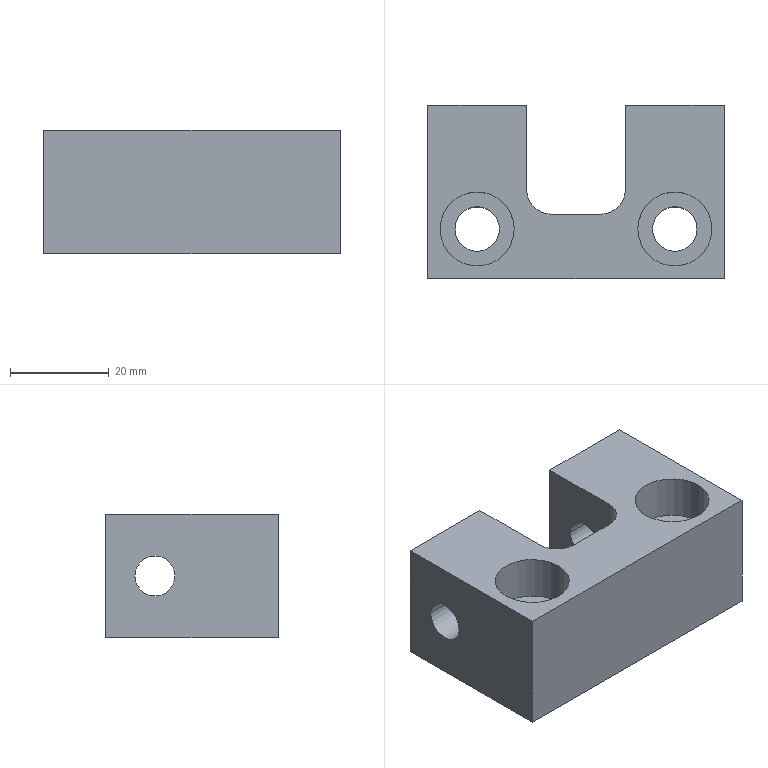Part | SolidWorks | features BaseBody 1 | 1 solid | 26 faces | box 60 x 35 x 25 mm | volume 34490 mm3 | cylinder 14 | plane 12 | commonest cylinder face diameters 8.1 x4 9 x4 15 x4 10 x2
STEP:
#1=CARTESIAN_POINT('',(-27.5,-7.5,16.));
#2=VERTEX_POINT('',#1);
#3=CARTESIAN_POINT('',(-12.5,-7.5,16.));
#4=VERTEX_POINT('',#3);
#5=CARTESIAN_POINT('',(-20.,-7.5,16.));
#6=DIRECTION('',(0.,0.,1.));
#7=DIRECTION('',(1.,0.,0.));
#8=AXIS2_PLACEMENT_3D('',#5,#6,#7);
#9=CIRCLE('',#8,7.5);
#10=EDGE_CURVE('',#2,#4,#9,.T.);
#11=ORIENTED_EDGE('',*,*,#10,.F.);
#12=CARTESIAN_POINT('',(-27.5,-7.5,25.));
#13=VERTEX_POINT('',#12);
#14=CARTESIAN_POINT('',(-27.5,-7.5,25.));
#15=DIRECTION('',(0.,0.,1.));
#16=VECTOR('',#15,1000.);
#17=LINE('',#14,#16);
#18=EDGE_CURVE('',#2,#13,#17,.T.);
#19=ORIENTED_EDGE('',*,*,#18,.T.);
#20=CARTESIAN_POINT('',(-12.5,-7.5,25.));
#21=VERTEX_POINT('',#20);
#22=CARTESIAN_POINT('',(-20.,-7.5,25.));
#23=DIRECTION('',(0.,0.,1.));
#24=DIRECTION('',(1.,0.,0.));
#25=AXIS2_PLACEMENT_3D('',#22,#23,#24);
#26=CIRCLE('',#25,7.5);
#27=EDGE_CURVE('',#13,#21,#26,.T.);
#28=ORIENTED_EDGE('',*,*,#27,.T.);
#29=CARTESIAN_POINT('',(-12.5,-7.5,25.));
#30=DIRECTION('',(0.,0.,1.));
#31=VECTOR('',#30,1000.);
#32=LINE('',#29,#31);
#33=EDGE_CURVE('',#4,#21,#32,.T.);
#34=ORIENTED_EDGE('',*,*,#33,.F.);
#35=EDGE_LOOP('',(#11,#19,#28,#34));
#36=FACE_OUTER_BOUND('',#35,.T.);
#37=CARTESIAN_POINT('',(-20.,-7.5,25.));
#38=DIRECTION('',(0.,0.,1.));
#39=DIRECTION('',(1.,0.,0.));
#40=AXIS2_PLACEMENT_3D('',#37,#38,#39);
#41=CYLINDRICAL_SURFACE('',#40,7.5);
#42=ADVANCED_FACE('',(#36),#41,.F.);
#43=CARTESIAN_POINT('',(-24.5,-7.5,0.));
#44=VERTEX_POINT('',#43);
#45=CARTESIAN_POINT('',(-15.5,-7.5,0.));
#46=VERTEX_POINT('',#45);
#47=CARTESIAN_POINT('',(-20.,-7.5,0.));
#48=DIRECTION('',(0.,0.,1.));
#49=DIRECTION('',(1.,0.,0.));
#50=AXIS2_PLACEMENT_3D('',#47,#48,#49);
#51=CIRCLE('',#50,4.5);
#52=EDGE_CURVE('',#44,#46,#51,.T.);
#53=ORIENTED_EDGE('',*,*,#52,.F.);
#54=CARTESIAN_POINT('',(-24.5,-7.5,16.));
#55=VERTEX_POINT('',#54);
#56=CARTESIAN_POINT('',(-24.5,-7.5,25.));
#57=DIRECTION('',(0.,0.,1.));
#58=VECTOR('',#57,1000.);
#59=LINE('',#56,#58);
#60=EDGE_CURVE('',#44,#55,#59,.T.);
#61=ORIENTED_EDGE('',*,*,#60,.T.);
#62=CARTESIAN_POINT('',(-15.5,-7.5,16.));
#63=VERTEX_POINT('',#62);
#64=CARTESIAN_POINT('',(-20.,-7.5,16.));
#65=DIRECTION('',(0.,0.,1.));
#66=DIRECTION('',(1.,0.,0.));
#67=AXIS2_PLACEMENT_3D('',#64,#65,#66);
#68=CIRCLE('',#67,4.5);
#69=EDGE_CURVE('',#55,#63,#68,.T.);
#70=ORIENTED_EDGE('',*,*,#69,.T.);
#71=CARTESIAN_POINT('',(-15.5,-7.5,25.));
#72=DIRECTION('',(0.,0.,1.));
#73=VECTOR('',#72,1000.);
#74=LINE('',#71,#73);
#75=EDGE_CURVE('',#46,#63,#74,.T.);
#76=ORIENTED_EDGE('',*,*,#75,.F.);
#77=EDGE_LOOP('',(#53,#61,#70,#76));
#78=FACE_OUTER_BOUND('',#77,.T.);
#79=CARTESIAN_POINT('',(-20.,-7.5,25.));
#80=DIRECTION('',(0.,0.,1.));
#81=DIRECTION('',(1.,0.,0.));
#82=AXIS2_PLACEMENT_3D('',#79,#80,#81);
#83=CYLINDRICAL_SURFACE('',#82,4.5);
#84=ADVANCED_FACE('',(#78),#83,.F.);
#85=CARTESIAN_POINT('',(12.5,-7.5,16.));
#86=VERTEX_POINT('',#85);
#87=CARTESIAN_POINT('',(27.5,-7.5,16.));
#88=VERTEX_POINT('',#87);
#89=CARTESIAN_POINT('',(20.,-7.5,16.));
#90=DIRECTION('',(0.,0.,1.));
#91=DIRECTION('',(1.,0.,0.));
#92=AXIS2_PLACEMENT_3D('',#89,#90,#91);
#93=CIRCLE('',#92,7.5);
#94=EDGE_CURVE('',#86,#88,#93,.T.);
#95=ORIENTED_EDGE('',*,*,#94,.F.);
#96=CARTESIAN_POINT('',(12.5,-7.5,25.));
#97=VERTEX_POINT('',#96);
#98=CARTESIAN_POINT('',(12.5,-7.5,25.));
#99=DIRECTION('',(0.,0.,1.));
#100=VECTOR('',#99,1000.);
#101=LINE('',#98,#100);
#102=EDGE_CURVE('',#86,#97,#101,.T.);
#103=ORIENTED_EDGE('',*,*,#102,.T.);
#104=CARTESIAN_POINT('',(27.5,-7.5,25.));
#105=VERTEX_POINT('',#104);
#106=CARTESIAN_POINT('',(20.,-7.5,25.));
#107=DIRECTION('',(0.,0.,1.));
#108=DIRECTION('',(1.,0.,0.));
#109=AXIS2_PLACEMENT_3D('',#106,#107,#108);
#110=CIRCLE('',#109,7.5);
#111=EDGE_CURVE('',#97,#105,#110,.T.);
#112=ORIENTED_EDGE('',*,*,#111,.T.);
#113=CARTESIAN_POINT('',(27.5,-7.5,25.));
#114=DIRECTION('',(0.,0.,1.));
#115=VECTOR('',#114,1000.);
#116=LINE('',#113,#115);
#117=EDGE_CURVE('',#88,#105,#116,.T.);
#118=ORIENTED_EDGE('',*,*,#117,.F.);
#119=EDGE_LOOP('',(#95,#103,#112,#118));
#120=FACE_OUTER_BOUND('',#119,.T.);
#121=CARTESIAN_POINT('',(20.,-7.5,25.));
#122=DIRECTION('',(0.,0.,1.));
#123=DIRECTION('',(1.,0.,0.));
#124=AXIS2_PLACEMENT_3D('',#121,#122,#123);
#125=CYLINDRICAL_SURFACE('',#124,7.5);
#126=ADVANCED_FACE('',(#120),#125,.F.);
#127=CARTESIAN_POINT('',(15.5,-7.5,0.));
#128=VERTEX_POINT('',#127);
#129=CARTESIAN_POINT('',(24.5,-7.5,0.));
#130=VERTEX_POINT('',#129);
#131=CARTESIAN_POINT('',(20.,-7.5,0.));
#132=DIRECTION('',(0.,0.,1.));
#133=DIRECTION('',(1.,0.,0.));
#134=AXIS2_PLACEMENT_3D('',#131,#132,#133);
#135=CIRCLE('',#134,4.5);
#136=EDGE_CURVE('',#128,#130,#135,.T.);
#137=ORIENTED_EDGE('',*,*,#136,.F.);
#138=CARTESIAN_POINT('',(15.5,-7.5,16.));
#139=VERTEX_POINT('',#138);
#140=CARTESIAN_POINT('',(15.5,-7.5,25.));
#141=DIRECTION('',(0.,0.,1.));
#142=VECTOR('',#141,1000.);
#143=LINE('',#140,#142);
#144=EDGE_CURVE('',#128,#139,#143,.T.);
#145=ORIENTED_EDGE('',*,*,#144,.T.);
#146=CARTESIAN_POINT('',(24.5,-7.5,16.));
#147=VERTEX_POINT('',#146);
#148=CARTESIAN_POINT('',(20.,-7.5,16.));
#149=DIRECTION('',(0.,0.,1.));
#150=DIRECTION('',(1.,0.,0.));
#151=AXIS2_PLACEMENT_3D('',#148,#149,#150);
#152=CIRCLE('',#151,4.5);
#153=EDGE_CURVE('',#139,#147,#152,.T.);
#154=ORIENTED_EDGE('',*,*,#153,.T.);
#155=CARTESIAN_POINT('',(24.5,-7.5,25.));
#156=DIRECTION('',(0.,0.,1.));
#157=VECTOR('',#156,1000.);
#158=LINE('',#155,#157);
#159=EDGE_CURVE('',#130,#147,#158,.T.);
#160=ORIENTED_EDGE('',*,*,#159,.F.);
#161=EDGE_LOOP('',(#137,#145,#154,#160));
#162=FACE_OUTER_BOUND('',#161,.T.);
#163=CARTESIAN_POINT('',(20.,-7.5,25.));
#164=DIRECTION('',(0.,0.,1.));
#165=DIRECTION('',(1.,0.,0.));
#166=AXIS2_PLACEMENT_3D('',#163,#164,#165);
#167=CYLINDRICAL_SURFACE('',#166,4.5);
#168=ADVANCED_FACE('',(#162),#167,.F.);
#169=CARTESIAN_POINT('',(-30.,3.45,12.5));
#170=VERTEX_POINT('',#169);
#171=CARTESIAN_POINT('',(-30.,11.55,12.5));
#172=VERTEX_POINT('',#171);
#173=CARTESIAN_POINT('',(-30.,7.5,12.5));
#174=DIRECTION('',(1.,0.,0.));
#175=DIRECTION('',(0.,1.,0.));
#176=AXIS2_PLACEMENT_3D('',#173,#174,#175);
#177=CIRCLE('',#176,4.05);
#178=EDGE_CURVE('',#170,#172,#177,.T.);
#179=ORIENTED_EDGE('',*,*,#178,.F.);
#180=CARTESIAN_POINT('',(-10.,3.45,12.5));
#181=VERTEX_POINT('',#180);
#182=CARTESIAN_POINT('',(-30.,3.45,12.5));
#183=DIRECTION('',(1.,0.,0.));
#184=VECTOR('',#183,1000.);
#185=LINE('',#182,#184);
#186=EDGE_CURVE('',#170,#181,#185,.T.);
#187=ORIENTED_EDGE('',*,*,#186,.T.);
#188=CARTESIAN_POINT('',(-10.,11.55,12.5));
#189=VERTEX_POINT('',#188);
#190=CARTESIAN_POINT('',(-10.,7.5,12.5));
#191=DIRECTION('',(1.,0.,0.));
#192=DIRECTION('',(0.,0.,1.));
#193=AXIS2_PLACEMENT_3D('',#190,#191,#192);
#194=CIRCLE('',#193,4.05);
#195=EDGE_CURVE('',#181,#189,#194,.T.);
#196=ORIENTED_EDGE('',*,*,#195,.T.);
#197=CARTESIAN_POINT('',(-30.,11.55,12.5));
#198=DIRECTION('',(1.,0.,0.));
#199=VECTOR('',#198,1000.);
#200=LINE('',#197,#199);
#201=EDGE_CURVE('',#172,#189,#200,.T.);
#202=ORIENTED_EDGE('',*,*,#201,.F.);
#203=EDGE_LOOP('',(#179,#187,#196,#202));
#204=FACE_OUTER_BOUND('',#203,.T.);
#205=CARTESIAN_POINT('',(-30.,7.5,12.5));
#206=DIRECTION('',(1.,0.,0.));
#207=DIRECTION('',(0.,1.,0.));
#208=AXIS2_PLACEMENT_3D('',#205,#206,#207);
#209=CYLINDRICAL_SURFACE('',#208,4.05);
#210=ADVANCED_FACE('',(#204),#209,.F.);
#211=CARTESIAN_POINT('',(10.,11.55,12.5));
#212=VERTEX_POINT('',#211);
#213=CARTESIAN_POINT('',(10.,3.45,12.5));
#214=VERTEX_POINT('',#213);
#215=CARTESIAN_POINT('',(10.,7.5,12.5));
#216=DIRECTION('',(-1.,0.,0.));
#217=DIRECTION('',(0.,1.,0.));
#218=AXIS2_PLACEMENT_3D('',#215,#216,#217);
#219=CIRCLE('',#218,4.05);
#220=EDGE_CURVE('',#212,#214,#219,.T.);
#221=ORIENTED_EDGE('',*,*,#220,.T.);
#222=CARTESIAN_POINT('',(30.,3.45,12.5));
#223=VERTEX_POINT('',#222);
#224=CARTESIAN_POINT('',(-30.,3.45,12.5));
#225=DIRECTION('',(1.,0.,0.));
#226=VECTOR('',#225,1000.);
#227=LINE('',#224,#226);
#228=EDGE_CURVE('',#214,#223,#227,.T.);
#229=ORIENTED_EDGE('',*,*,#228,.T.);
#230=CARTESIAN_POINT('',(30.,11.55,12.5));
#231=VERTEX_POINT('',#230);
#232=CARTESIAN_POINT('',(30.,7.5,12.5));
#233=DIRECTION('',(1.,0.,0.));
#234=DIRECTION('',(0.,1.,0.));
#235=AXIS2_PLACEMENT_3D('',#232,#233,#234);
#236=CIRCLE('',#235,4.05);
#237=EDGE_CURVE('',#223,#231,#236,.T.);
#238=ORIENTED_EDGE('',*,*,#237,.T.);
#239=CARTESIAN_POINT('',(-30.,11.55,12.5));
#240=DIRECTION('',(1.,0.,0.));
#241=VECTOR('',#240,1000.);
#242=LINE('',#239,#241);
#243=EDGE_CURVE('',#212,#231,#242,.T.);
#244=ORIENTED_EDGE('',*,*,#243,.F.);
#245=EDGE_LOOP('',(#221,#229,#238,#244));
#246=FACE_OUTER_BOUND('',#245,.T.);
#247=CARTESIAN_POINT('',(-30.,7.5,12.5));
#248=DIRECTION('',(1.,0.,0.));
#249=DIRECTION('',(0.,1.,0.));
#250=AXIS2_PLACEMENT_3D('',#247,#248,#249);
#251=CYLINDRICAL_SURFACE('',#250,4.05);
#252=ADVANCED_FACE('',(#246),#251,.F.);
#253=CARTESIAN_POINT('',(-10.,0.5,0.));
#254=VERTEX_POINT('',#253);
#255=CARTESIAN_POINT('',(-5.,-4.5,0.));
#256=VERTEX_POINT('',#255);
#257=CARTESIAN_POINT('',(-5.,0.5,0.));
#258=DIRECTION('',(0.,0.,1.));
#259=DIRECTION('',(1.,0.,0.));
#260=AXIS2_PLACEMENT_3D('',#257,#258,#259);
#261=CIRCLE('',#260,5.);
#262=EDGE_CURVE('',#254,#256,#261,.T.);
#263=ORIENTED_EDGE('',*,*,#262,.F.);
#264=CARTESIAN_POINT('',(-10.,0.5,25.));
#265=VERTEX_POINT('',#264);
#266=CARTESIAN_POINT('',(-10.,0.5,0.));
#267=DIRECTION('',(0.,0.,-1.));
#268=VECTOR('',#267,1000.);
#269=LINE('',#266,#268);
#270=EDGE_CURVE('',#265,#254,#269,.T.);
#271=ORIENTED_EDGE('',*,*,#270,.F.);
#272=CARTESIAN_POINT('',(-5.,-4.5,25.));
#273=VERTEX_POINT('',#272);
#274=CARTESIAN_POINT('',(-5.,0.5,25.));
#275=DIRECTION('',(0.,0.,-1.));
#276=DIRECTION('',(1.,0.,0.));
#277=AXIS2_PLACEMENT_3D('',#274,#275,#276);
#278=CIRCLE('',#277,5.);
#279=EDGE_CURVE('',#273,#265,#278,.T.);
#280=ORIENTED_EDGE('',*,*,#279,.F.);
#281=CARTESIAN_POINT('',(-5.,-4.5,25.));
#282=DIRECTION('',(0.,0.,1.));
#283=VECTOR('',#282,1000.);
#284=LINE('',#281,#283);
#285=EDGE_CURVE('',#256,#273,#284,.T.);
#286=ORIENTED_EDGE('',*,*,#285,.F.);
#287=EDGE_LOOP('',(#263,#271,#280,#286));
#288=FACE_OUTER_BOUND('',#287,.T.);
#289=CARTESIAN_POINT('',(-5.,0.5,0.));
#290=DIRECTION('',(0.,0.,-1.));
#291=DIRECTION('',(-1.,0.,0.));
#292=AXIS2_PLACEMENT_3D('',#289,#290,#291);
#293=CYLINDRICAL_SURFACE('',#292,5.);
#294=ADVANCED_FACE('',(#288),#293,.F.);
#295=CARTESIAN_POINT('',(5.,-4.5,0.));
#296=VERTEX_POINT('',#295);
#297=CARTESIAN_POINT('',(10.,0.5,0.));
#298=VERTEX_POINT('',#297);
#299=CARTESIAN_POINT('',(5.,0.5,0.));
#300=DIRECTION('',(0.,0.,1.));
#301=DIRECTION('',(1.,0.,0.));
#302=AXIS2_PLACEMENT_3D('',#299,#300,#301);
#303=CIRCLE('',#302,5.);
#304=EDGE_CURVE('',#296,#298,#303,.T.);
#305=ORIENTED_EDGE('',*,*,#304,.F.);
#306=CARTESIAN_POINT('',(5.,-4.5,25.));
#307=VERTEX_POINT('',#306);
#308=CARTESIAN_POINT('',(5.,-4.5,0.));
#309=DIRECTION('',(0.,0.,-1.));
#310=VECTOR('',#309,1000.);
#311=LINE('',#308,#310);
#312=EDGE_CURVE('',#307,#296,#311,.T.);
#313=ORIENTED_EDGE('',*,*,#312,.F.);
#314=CARTESIAN_POINT('',(10.,0.5,25.));
#315=VERTEX_POINT('',#314);
#316=CARTESIAN_POINT('',(5.,0.5,25.));
#317=DIRECTION('',(0.,0.,-1.));
#318=DIRECTION('',(1.,0.,0.));
#319=AXIS2_PLACEMENT_3D('',#316,#317,#318);
#320=CIRCLE('',#319,5.);
#321=EDGE_CURVE('',#315,#307,#320,.T.);
#322=ORIENTED_EDGE('',*,*,#321,.F.);
#323=CARTESIAN_POINT('',(10.,0.5,25.));
#324=DIRECTION('',(0.,0.,1.));
#325=VECTOR('',#324,1000.);
#326=LINE('',#323,#325);
#327=EDGE_CURVE('',#298,#315,#326,.T.);
#328=ORIENTED_EDGE('',*,*,#327,.F.);
#329=EDGE_LOOP('',(#305,#313,#322,#328));
#330=FACE_OUTER_BOUND('',#329,.T.);
#331=CARTESIAN_POINT('',(5.,0.5,0.));
#332=DIRECTION('',(0.,0.,-1.));
#333=DIRECTION('',(-1.,0.,0.));
#334=AXIS2_PLACEMENT_3D('',#331,#332,#333);
#335=CYLINDRICAL_SURFACE('',#334,5.);
#336=ADVANCED_FACE('',(#330),#335,.F.);
#337=CARTESIAN_POINT('',(-10.,-4.5,25.));
#338=DIRECTION('',(1.,0.,0.));
#339=VECTOR('',#338,1000.);
#340=LINE('',#337,#339);
#341=EDGE_CURVE('',#273,#307,#340,.T.);
#342=ORIENTED_EDGE('',*,*,#341,.T.);
#343=ORIENTED_EDGE('',*,*,#312,.T.);
#344=CARTESIAN_POINT('',(-10.,-4.5,0.));
#345=DIRECTION('',(1.,0.,0.));
#346=VECTOR('',#345,1000.);
#347=LINE('',#344,#346);
#348=EDGE_CURVE('',#256,#296,#347,.T.);
#349=ORIENTED_EDGE('',*,*,#348,.F.);
#350=ORIENTED_EDGE('',*,*,#285,.T.);
#351=EDGE_LOOP('',(#342,#343,#349,#350));
#352=FACE_OUTER_BOUND('',#351,.T.);
#353=CARTESIAN_POINT('',(-10.,-4.5,0.));
#354=DIRECTION('',(0.,-1.,0.));
#355=DIRECTION('',(-1.,0.,0.));
#356=AXIS2_PLACEMENT_3D('',#353,#354,#355);
#357=PLANE('',#356);
#358=ADVANCED_FACE('',(#352),#357,.F.);
#359=CARTESIAN_POINT('',(-10.,7.5,12.5));
#360=DIRECTION('',(1.,0.,0.));
#361=DIRECTION('',(0.,0.,1.));
#362=AXIS2_PLACEMENT_3D('',#359,#360,#361);
#363=CIRCLE('',#362,4.05);
#364=EDGE_CURVE('',#189,#181,#363,.T.);
#365=ORIENTED_EDGE('',*,*,#364,.F.);
#366=ORIENTED_EDGE('',*,*,#195,.F.);
#367=EDGE_LOOP('',(#365,#366));
#368=FACE_BOUND('',#367,.T.);
#369=CARTESIAN_POINT('',(-10.,17.5,25.));
#370=VERTEX_POINT('',#369);
#371=CARTESIAN_POINT('',(-10.,39.5,25.));
#372=DIRECTION('',(0.,-1.,0.));
#373=VECTOR('',#372,1000.);
#374=LINE('',#371,#373);
#375=EDGE_CURVE('',#370,#265,#374,.T.);
#376=ORIENTED_EDGE('',*,*,#375,.T.);
#377=ORIENTED_EDGE('',*,*,#270,.T.);
#378=CARTESIAN_POINT('',(-10.,17.5,0.));
#379=VERTEX_POINT('',#378);
#380=CARTESIAN_POINT('',(-10.,39.5,0.));
#381=DIRECTION('',(0.,-1.,0.));
#382=VECTOR('',#381,1000.);
#383=LINE('',#380,#382);
#384=EDGE_CURVE('',#379,#254,#383,.T.);
#385=ORIENTED_EDGE('',*,*,#384,.F.);
#386=CARTESIAN_POINT('',(-10.,17.5,25.));
#387=DIRECTION('',(0.,0.,-1.));
#388=VECTOR('',#387,1000.);
#389=LINE('',#386,#388);
#390=EDGE_CURVE('',#370,#379,#389,.T.);
#391=ORIENTED_EDGE('',*,*,#390,.F.);
#392=EDGE_LOOP('',(#376,#377,#385,#391));
#393=FACE_OUTER_BOUND('',#392,.T.);
#394=CARTESIAN_POINT('',(-10.,39.5,0.));
#395=DIRECTION('',(-1.,0.,0.));
#396=DIRECTION('',(0.,0.,1.));
#397=AXIS2_PLACEMENT_3D('',#394,#395,#396);
#398=PLANE('',#397);
#399=ADVANCED_FACE('',(#368,#393),#398,.F.);
#400=ORIENTED_EDGE('',*,*,#220,.F.);
#401=CARTESIAN_POINT('',(10.,7.5,12.5));
#402=DIRECTION('',(-1.,0.,0.));
#403=DIRECTION('',(0.,1.,0.));
#404=AXIS2_PLACEMENT_3D('',#401,#402,#403);
#405=CIRCLE('',#404,4.05);
#406=EDGE_CURVE('',#214,#212,#405,.T.);
#407=ORIENTED_EDGE('',*,*,#406,.F.);
#408=EDGE_LOOP('',(#400,#407));
#409=FACE_BOUND('',#408,.T.);
#410=CARTESIAN_POINT('',(10.,17.5,0.));
#411=VERTEX_POINT('',#410);
#412=CARTESIAN_POINT('',(10.,39.5,0.));
#413=DIRECTION('',(0.,1.,0.));
#414=VECTOR('',#413,1000.);
#415=LINE('',#412,#414);
#416=EDGE_CURVE('',#298,#411,#415,.T.);
#417=ORIENTED_EDGE('',*,*,#416,.F.);
#418=ORIENTED_EDGE('',*,*,#327,.T.);
#419=CARTESIAN_POINT('',(10.,17.5,25.));
#420=VERTEX_POINT('',#419);
#421=CARTESIAN_POINT('',(10.,39.5,25.));
#422=DIRECTION('',(0.,1.,0.));
#423=VECTOR('',#422,1000.);
#424=LINE('',#421,#423);
#425=EDGE_CURVE('',#315,#420,#424,.T.);
#426=ORIENTED_EDGE('',*,*,#425,.T.);
#427=CARTESIAN_POINT('',(10.,17.5,25.));
#428=DIRECTION('',(0.,0.,1.));
#429=VECTOR('',#428,1000.);
#430=LINE('',#427,#429);
#431=EDGE_CURVE('',#411,#420,#430,.T.);
#432=ORIENTED_EDGE('',*,*,#431,.F.);
#433=EDGE_LOOP('',(#417,#418,#426,#432));
#434=FACE_OUTER_BOUND('',#433,.T.);
#435=CARTESIAN_POINT('',(10.,39.5,0.));
#436=DIRECTION('',(1.,0.,0.));
#437=DIRECTION('',(0.,1.,0.));
#438=AXIS2_PLACEMENT_3D('',#435,#436,#437);
#439=PLANE('',#438);
#440=ADVANCED_FACE('',(#409,#434),#439,.F.);
#441=CARTESIAN_POINT('',(-20.,-7.5,16.));
#442=DIRECTION('',(0.,0.,1.));
#443=DIRECTION('',(1.,0.,0.));
#444=AXIS2_PLACEMENT_3D('',#441,#442,#443);
#445=CIRCLE('',#444,4.5);
#446=EDGE_CURVE('',#63,#55,#445,.T.);
#447=ORIENTED_EDGE('',*,*,#446,.F.);
#448=ORIENTED_EDGE('',*,*,#69,.F.);
#449=EDGE_LOOP('',(#447,#448));
#450=FACE_BOUND('',#449,.T.);
#451=CARTESIAN_POINT('',(-20.,-7.5,16.));
#452=DIRECTION('',(0.,0.,1.));
#453=DIRECTION('',(1.,0.,0.));
#454=AXIS2_PLACEMENT_3D('',#451,#452,#453);
#455=CIRCLE('',#454,7.5);
#456=EDGE_CURVE('',#4,#2,#455,.T.);
#457=ORIENTED_EDGE('',*,*,#456,.T.);
#458=ORIENTED_EDGE('',*,*,#10,.T.);
#459=EDGE_LOOP('',(#457,#458));
#460=FACE_OUTER_BOUND('',#459,.T.);
#461=CARTESIAN_POINT('',(-15.5,-7.5,16.));
#462=DIRECTION('',(0.,0.,-1.));
#463=DIRECTION('',(0.,-1.,0.));
#464=AXIS2_PLACEMENT_3D('',#461,#462,#463);
#465=PLANE('',#464);
#466=ADVANCED_FACE('',(#450,#460),#465,.F.);
#467=CARTESIAN_POINT('',(20.,-7.5,16.));
#468=DIRECTION('',(0.,0.,1.));
#469=DIRECTION('',(1.,0.,0.));
#470=AXIS2_PLACEMENT_3D('',#467,#468,#469);
#471=CIRCLE('',#470,4.5);
#472=EDGE_CURVE('',#147,#139,#471,.T.);
#473=ORIENTED_EDGE('',*,*,#472,.F.);
#474=ORIENTED_EDGE('',*,*,#153,.F.);
#475=EDGE_LOOP('',(#473,#474));
#476=FACE_BOUND('',#475,.T.);
#477=CARTESIAN_POINT('',(20.,-7.5,16.));
#478=DIRECTION('',(0.,0.,1.));
#479=DIRECTION('',(1.,0.,0.));
#480=AXIS2_PLACEMENT_3D('',#477,#478,#479);
#481=CIRCLE('',#480,7.5);
#482=EDGE_CURVE('',#88,#86,#481,.T.);
#483=ORIENTED_EDGE('',*,*,#482,.T.);
#484=ORIENTED_EDGE('',*,*,#94,.T.);
#485=EDGE_LOOP('',(#483,#484));
#486=FACE_OUTER_BOUND('',#485,.T.);
#487=CARTESIAN_POINT('',(24.5,-7.5,16.));
#488=DIRECTION('',(0.,0.,-1.));
#489=DIRECTION('',(0.,-1.,0.));
#490=AXIS2_PLACEMENT_3D('',#487,#488,#489);
#491=PLANE('',#490);
#492=ADVANCED_FACE('',(#476,#486),#491,.F.);
#493=CARTESIAN_POINT('',(20.,-7.5,0.));
#494=DIRECTION('',(0.,0.,1.));
#495=DIRECTION('',(1.,0.,0.));
#496=AXIS2_PLACEMENT_3D('',#493,#494,#495);
#497=CIRCLE('',#496,4.5);
#498=EDGE_CURVE('',#130,#128,#497,.T.);
#499=ORIENTED_EDGE('',*,*,#498,.T.);
#500=ORIENTED_EDGE('',*,*,#136,.T.);
#501=EDGE_LOOP('',(#499,#500));
#502=FACE_BOUND('',#501,.T.);
#503=CARTESIAN_POINT('',(-20.,-7.5,0.));
#504=DIRECTION('',(0.,0.,1.));
#505=DIRECTION('',(1.,0.,0.));
#506=AXIS2_PLACEMENT_3D('',#503,#504,#505);
#507=CIRCLE('',#506,4.5);
#508=EDGE_CURVE('',#46,#44,#507,.T.);
#509=ORIENTED_EDGE('',*,*,#508,.T.);
#510=ORIENTED_EDGE('',*,*,#52,.T.);
#511=EDGE_LOOP('',(#509,#510));
#512=FACE_BOUND('',#511,.T.);
#513=ORIENTED_EDGE('',*,*,#384,.T.);
#514=ORIENTED_EDGE('',*,*,#262,.T.);
#515=ORIENTED_EDGE('',*,*,#348,.T.);
#516=ORIENTED_EDGE('',*,*,#304,.T.);
#517=ORIENTED_EDGE('',*,*,#416,.T.);
#518=CARTESIAN_POINT('',(30.,17.5,0.));
#519=VERTEX_POINT('',#518);
#520=CARTESIAN_POINT('',(-30.,17.5,0.));
#521=DIRECTION('',(-1.,0.,0.));
#522=VECTOR('',#521,1000.);
#523=LINE('',#520,#522);
#524=EDGE_CURVE('',#519,#411,#523,.T.);
#525=ORIENTED_EDGE('',*,*,#524,.F.);
#526=CARTESIAN_POINT('',(30.,-17.5,0.));
#527=VERTEX_POINT('',#526);
#528=CARTESIAN_POINT('',(30.,17.5,0.));
#529=DIRECTION('',(0.,1.,0.));
#530=VECTOR('',#529,1000.);
#531=LINE('',#528,#530);
#532=EDGE_CURVE('',#527,#519,#531,.T.);
#533=ORIENTED_EDGE('',*,*,#532,.F.);
#534=CARTESIAN_POINT('',(-30.,-17.5,0.));
#535=VERTEX_POINT('',#534);
#536=CARTESIAN_POINT('',(-30.,-17.5,0.));
#537=DIRECTION('',(1.,0.,0.));
#538=VECTOR('',#537,1000.);
#539=LINE('',#536,#538);
#540=EDGE_CURVE('',#535,#527,#539,.T.);
#541=ORIENTED_EDGE('',*,*,#540,.F.);
#542=CARTESIAN_POINT('',(-30.,17.5,0.));
#543=VERTEX_POINT('',#542);
#544=CARTESIAN_POINT('',(-30.,17.5,0.));
#545=DIRECTION('',(0.,-1.,0.));
#546=VECTOR('',#545,1000.);
#547=LINE('',#544,#546);
#548=EDGE_CURVE('',#543,#535,#547,.T.);
#549=ORIENTED_EDGE('',*,*,#548,.F.);
#550=CARTESIAN_POINT('',(-30.,17.5,0.));
#551=DIRECTION('',(-1.,0.,0.));
#552=VECTOR('',#551,1000.);
#553=LINE('',#550,#552);
#554=EDGE_CURVE('',#379,#543,#553,.T.);
#555=ORIENTED_EDGE('',*,*,#554,.F.);
#556=EDGE_LOOP('',(#513,#514,#515,#516,#517,#525,#533,#541,#549,#555));
#557=FACE_OUTER_BOUND('',#556,.T.);
#558=CARTESIAN_POINT('',(0.,0.,0.));
#559=DIRECTION('',(0.,0.,1.));
#560=DIRECTION('',(1.,0.,0.));
#561=AXIS2_PLACEMENT_3D('',#558,#559,#560);
#562=PLANE('',#561);
#563=ADVANCED_FACE('',(#502,#512,#557),#562,.F.);
#564=CARTESIAN_POINT('',(20.,-7.5,25.));
#565=DIRECTION('',(0.,0.,1.));
#566=DIRECTION('',(1.,0.,0.));
#567=AXIS2_PLACEMENT_3D('',#564,#565,#566);
#568=CIRCLE('',#567,7.5);
#569=EDGE_CURVE('',#105,#97,#568,.T.);
#570=ORIENTED_EDGE('',*,*,#569,.F.);
#571=ORIENTED_EDGE('',*,*,#111,.F.);
#572=EDGE_LOOP('',(#570,#571));
#573=FACE_BOUND('',#572,.T.);
#574=CARTESIAN_POINT('',(-20.,-7.5,25.));
#575=DIRECTION('',(0.,0.,1.));
#576=DIRECTION('',(1.,0.,0.));
#577=AXIS2_PLACEMENT_3D('',#574,#575,#576);
#578=CIRCLE('',#577,7.5);
#579=EDGE_CURVE('',#21,#13,#578,.T.);
#580=ORIENTED_EDGE('',*,*,#579,.F.);
#581=ORIENTED_EDGE('',*,*,#27,.F.);
#582=EDGE_LOOP('',(#580,#581));
#583=FACE_BOUND('',#582,.T.);
#584=ORIENTED_EDGE('',*,*,#425,.F.);
#585=ORIENTED_EDGE('',*,*,#321,.T.);
#586=ORIENTED_EDGE('',*,*,#341,.F.);
#587=ORIENTED_EDGE('',*,*,#279,.T.);
#588=ORIENTED_EDGE('',*,*,#375,.F.);
#589=CARTESIAN_POINT('',(-30.,17.5,25.));
#590=VERTEX_POINT('',#589);
#591=CARTESIAN_POINT('',(-30.,17.5,25.));
#592=DIRECTION('',(-1.,0.,0.));
#593=VECTOR('',#592,1000.);
#594=LINE('',#591,#593);
#595=EDGE_CURVE('',#370,#590,#594,.T.);
#596=ORIENTED_EDGE('',*,*,#595,.T.);
#597=CARTESIAN_POINT('',(-30.,-17.5,25.));
#598=VERTEX_POINT('',#597);
#599=CARTESIAN_POINT('',(-30.,17.5,25.));
#600=DIRECTION('',(0.,-1.,0.));
#601=VECTOR('',#600,1000.);
#602=LINE('',#599,#601);
#603=EDGE_CURVE('',#590,#598,#602,.T.);
#604=ORIENTED_EDGE('',*,*,#603,.T.);
#605=CARTESIAN_POINT('',(30.,-17.5,25.));
#606=VERTEX_POINT('',#605);
#607=CARTESIAN_POINT('',(-30.,-17.5,25.));
#608=DIRECTION('',(1.,0.,0.));
#609=VECTOR('',#608,1000.);
#610=LINE('',#607,#609);
#611=EDGE_CURVE('',#598,#606,#610,.T.);
#612=ORIENTED_EDGE('',*,*,#611,.T.);
#613=CARTESIAN_POINT('',(30.,17.5,25.));
#614=VERTEX_POINT('',#613);
#615=CARTESIAN_POINT('',(30.,17.5,25.));
#616=DIRECTION('',(0.,1.,0.));
#617=VECTOR('',#616,1000.);
#618=LINE('',#615,#617);
#619=EDGE_CURVE('',#606,#614,#618,.T.);
#620=ORIENTED_EDGE('',*,*,#619,.T.);
#621=CARTESIAN_POINT('',(-30.,17.5,25.));
#622=DIRECTION('',(-1.,0.,0.));
#623=VECTOR('',#622,1000.);
#624=LINE('',#621,#623);
#625=EDGE_CURVE('',#614,#420,#624,.T.);
#626=ORIENTED_EDGE('',*,*,#625,.T.);
#627=EDGE_LOOP('',(#584,#585,#586,#587,#588,#596,#604,#612,#620,#626));
#628=FACE_OUTER_BOUND('',#627,.T.);
#629=CARTESIAN_POINT('',(0.,0.,25.));
#630=DIRECTION('',(0.,0.,1.));
#631=DIRECTION('',(1.,0.,0.));
#632=AXIS2_PLACEMENT_3D('',#629,#630,#631);
#633=PLANE('',#632);
#634=ADVANCED_FACE('',(#573,#583,#628),#633,.T.);
#635=ORIENTED_EDGE('',*,*,#540,.T.);
#636=CARTESIAN_POINT('',(30.,-17.5,25.));
#637=DIRECTION('',(0.,0.,-1.));
#638=VECTOR('',#637,1000.);
#639=LINE('',#636,#638);
#640=EDGE_CURVE('',#606,#527,#639,.T.);
#641=ORIENTED_EDGE('',*,*,#640,.F.);
#642=ORIENTED_EDGE('',*,*,#611,.F.);
#643=CARTESIAN_POINT('',(-30.,-17.5,25.));
#644=DIRECTION('',(0.,0.,-1.));
#645=VECTOR('',#644,1000.);
#646=LINE('',#643,#645);
#647=EDGE_CURVE('',#598,#535,#646,.T.);
#648=ORIENTED_EDGE('',*,*,#647,.T.);
#649=EDGE_LOOP('',(#635,#641,#642,#648));
#650=FACE_OUTER_BOUND('',#649,.T.);
#651=CARTESIAN_POINT('',(-30.,-17.5,25.));
#652=DIRECTION('',(0.,1.,0.));
#653=DIRECTION('',(1.,0.,0.));
#654=AXIS2_PLACEMENT_3D('',#651,#652,#653);
#655=PLANE('',#654);
#656=ADVANCED_FACE('',(#650),#655,.F.);
#657=CARTESIAN_POINT('',(-30.,7.5,12.5));
#658=DIRECTION('',(1.,0.,0.));
#659=DIRECTION('',(0.,1.,0.));
#660=AXIS2_PLACEMENT_3D('',#657,#658,#659);
#661=CIRCLE('',#660,4.05);
#662=EDGE_CURVE('',#172,#170,#661,.T.);
#663=ORIENTED_EDGE('',*,*,#662,.T.);
#664=ORIENTED_EDGE('',*,*,#178,.T.);
#665=EDGE_LOOP('',(#663,#664));
#666=FACE_BOUND('',#665,.T.);
#667=ORIENTED_EDGE('',*,*,#548,.T.);
#668=ORIENTED_EDGE('',*,*,#647,.F.);
#669=ORIENTED_EDGE('',*,*,#603,.F.);
#670=CARTESIAN_POINT('',(-30.,17.5,25.));
#671=DIRECTION('',(0.,0.,-1.));
#672=VECTOR('',#671,1000.);
#673=LINE('',#670,#672);
#674=EDGE_CURVE('',#590,#543,#673,.T.);
#675=ORIENTED_EDGE('',*,*,#674,.T.);
#676=EDGE_LOOP('',(#667,#668,#669,#675));
#677=FACE_OUTER_BOUND('',#676,.T.);
#678=CARTESIAN_POINT('',(-30.,17.5,25.));
#679=DIRECTION('',(1.,0.,0.));
#680=DIRECTION('',(0.,1.,0.));
#681=AXIS2_PLACEMENT_3D('',#678,#679,#680);
#682=PLANE('',#681);
#683=ADVANCED_FACE('',(#666,#677),#682,.F.);
#684=ORIENTED_EDGE('',*,*,#595,.F.);
#685=ORIENTED_EDGE('',*,*,#390,.T.);
#686=ORIENTED_EDGE('',*,*,#554,.T.);
#687=ORIENTED_EDGE('',*,*,#674,.F.);
#688=EDGE_LOOP('',(#684,#685,#686,#687));
#689=FACE_OUTER_BOUND('',#688,.T.);
#690=CARTESIAN_POINT('',(-30.,17.5,25.));
#691=DIRECTION('',(0.,-1.,0.));
#692=DIRECTION('',(0.,0.,-1.));
#693=AXIS2_PLACEMENT_3D('',#690,#691,#692);
#694=PLANE('',#693);
#695=ADVANCED_FACE('',(#689),#694,.F.);
#696=CARTESIAN_POINT('',(30.,7.5,12.5));
#697=DIRECTION('',(1.,0.,0.));
#698=DIRECTION('',(0.,1.,0.));
#699=AXIS2_PLACEMENT_3D('',#696,#697,#698);
#700=CIRCLE('',#699,4.05);
#701=EDGE_CURVE('',#231,#223,#700,.T.);
#702=ORIENTED_EDGE('',*,*,#701,.F.);
#703=ORIENTED_EDGE('',*,*,#237,.F.);
#704=EDGE_LOOP('',(#702,#703));
#705=FACE_BOUND('',#704,.T.);
#706=ORIENTED_EDGE('',*,*,#532,.T.);
#707=CARTESIAN_POINT('',(30.,17.5,25.));
#708=DIRECTION('',(0.,0.,-1.));
#709=VECTOR('',#708,1000.);
#710=LINE('',#707,#709);
#711=EDGE_CURVE('',#614,#519,#710,.T.);
#712=ORIENTED_EDGE('',*,*,#711,.F.);
#713=ORIENTED_EDGE('',*,*,#619,.F.);
#714=ORIENTED_EDGE('',*,*,#640,.T.);
#715=EDGE_LOOP('',(#706,#712,#713,#714));
#716=FACE_OUTER_BOUND('',#715,.T.);
#717=CARTESIAN_POINT('',(30.,17.5,25.));
#718=DIRECTION('',(-1.,0.,0.));
#719=DIRECTION('',(0.,1.,0.));
#720=AXIS2_PLACEMENT_3D('',#717,#718,#719);
#721=PLANE('',#720);
#722=ADVANCED_FACE('',(#705,#716),#721,.F.);
#723=ORIENTED_EDGE('',*,*,#524,.T.);
#724=ORIENTED_EDGE('',*,*,#431,.T.);
#725=ORIENTED_EDGE('',*,*,#625,.F.);
#726=ORIENTED_EDGE('',*,*,#711,.T.);
#727=EDGE_LOOP('',(#723,#724,#725,#726));
#728=FACE_OUTER_BOUND('',#727,.T.);
#729=CARTESIAN_POINT('',(-30.,17.5,25.));
#730=DIRECTION('',(0.,-1.,0.));
#731=DIRECTION('',(0.,0.,-1.));
#732=AXIS2_PLACEMENT_3D('',#729,#730,#731);
#733=PLANE('',#732);
#734=ADVANCED_FACE('',(#728),#733,.F.);
#735=ORIENTED_EDGE('',*,*,#228,.F.);
#736=ORIENTED_EDGE('',*,*,#406,.T.);
#737=ORIENTED_EDGE('',*,*,#243,.T.);
#738=ORIENTED_EDGE('',*,*,#701,.T.);
#739=EDGE_LOOP('',(#735,#736,#737,#738));
#740=FACE_OUTER_BOUND('',#739,.T.);
#741=CARTESIAN_POINT('',(-30.,7.5,12.5));
#742=DIRECTION('',(1.,0.,0.));
#743=DIRECTION('',(0.,1.,0.));
#744=AXIS2_PLACEMENT_3D('',#741,#742,#743);
#745=CYLINDRICAL_SURFACE('',#744,4.05);
#746=ADVANCED_FACE('',(#740),#745,.F.);
#747=ORIENTED_EDGE('',*,*,#186,.F.);
#748=ORIENTED_EDGE('',*,*,#662,.F.);
#749=ORIENTED_EDGE('',*,*,#201,.T.);
#750=ORIENTED_EDGE('',*,*,#364,.T.);
#751=EDGE_LOOP('',(#747,#748,#749,#750));
#752=FACE_OUTER_BOUND('',#751,.T.);
#753=CARTESIAN_POINT('',(-30.,7.5,12.5));
#754=DIRECTION('',(1.,0.,0.));
#755=DIRECTION('',(0.,1.,0.));
#756=AXIS2_PLACEMENT_3D('',#753,#754,#755);
#757=CYLINDRICAL_SURFACE('',#756,4.05);
#758=ADVANCED_FACE('',(#752),#757,.F.);
#759=ORIENTED_EDGE('',*,*,#144,.F.);
#760=ORIENTED_EDGE('',*,*,#498,.F.);
#761=ORIENTED_EDGE('',*,*,#159,.T.);
#762=ORIENTED_EDGE('',*,*,#472,.T.);
#763=EDGE_LOOP('',(#759,#760,#761,#762));
#764=FACE_OUTER_BOUND('',#763,.T.);
#765=CARTESIAN_POINT('',(20.,-7.5,25.));
#766=DIRECTION('',(0.,0.,1.));
#767=DIRECTION('',(1.,0.,0.));
#768=AXIS2_PLACEMENT_3D('',#765,#766,#767);
#769=CYLINDRICAL_SURFACE('',#768,4.5);
#770=ADVANCED_FACE('',(#764),#769,.F.);
#771=ORIENTED_EDGE('',*,*,#102,.F.);
#772=ORIENTED_EDGE('',*,*,#482,.F.);
#773=ORIENTED_EDGE('',*,*,#117,.T.);
#774=ORIENTED_EDGE('',*,*,#569,.T.);
#775=EDGE_LOOP('',(#771,#772,#773,#774));
#776=FACE_OUTER_BOUND('',#775,.T.);
#777=CARTESIAN_POINT('',(20.,-7.5,25.));
#778=DIRECTION('',(0.,0.,1.));
#779=DIRECTION('',(1.,0.,0.));
#780=AXIS2_PLACEMENT_3D('',#777,#778,#779);
#781=CYLINDRICAL_SURFACE('',#780,7.5);
#782=ADVANCED_FACE('',(#776),#781,.F.);
#783=ORIENTED_EDGE('',*,*,#60,.F.);
#784=ORIENTED_EDGE('',*,*,#508,.F.);
#785=ORIENTED_EDGE('',*,*,#75,.T.);
#786=ORIENTED_EDGE('',*,*,#446,.T.);
#787=EDGE_LOOP('',(#783,#784,#785,#786));
#788=FACE_OUTER_BOUND('',#787,.T.);
#789=CARTESIAN_POINT('',(-20.,-7.5,25.));
#790=DIRECTION('',(0.,0.,1.));
#791=DIRECTION('',(1.,0.,0.));
#792=AXIS2_PLACEMENT_3D('',#789,#790,#791);
#793=CYLINDRICAL_SURFACE('',#792,4.5);
#794=ADVANCED_FACE('',(#788),#793,.F.);
#795=ORIENTED_EDGE('',*,*,#18,.F.);
#796=ORIENTED_EDGE('',*,*,#456,.F.);
#797=ORIENTED_EDGE('',*,*,#33,.T.);
#798=ORIENTED_EDGE('',*,*,#579,.T.);
#799=EDGE_LOOP('',(#795,#796,#797,#798));
#800=FACE_OUTER_BOUND('',#799,.T.);
#801=CARTESIAN_POINT('',(-20.,-7.5,25.));
#802=DIRECTION('',(0.,0.,1.));
#803=DIRECTION('',(1.,0.,0.));
#804=AXIS2_PLACEMENT_3D('',#801,#802,#803);
#805=CYLINDRICAL_SURFACE('',#804,7.5);
#806=ADVANCED_FACE('',(#800),#805,.F.);
#807=CLOSED_SHELL('',(#42,#84,#126,#168,#210,#252,#294,#336,#358,#399,#440,#466,#492,#563,#634,#656,#683,#695,#722,#734,#746,#758,#770,#782,#794,#806));
#808=MANIFOLD_SOLID_BREP('',#807);
#809=CARTESIAN_POINT('',(0.,0.,0.));
#810=DIRECTION('',(0.,0.,1.));
#811=DIRECTION('',(1.,0.,0.));
#812=AXIS2_PLACEMENT_3D('',#809,#810,#811);
#813=(LENGTH_UNIT()NAMED_UNIT(*)SI_UNIT(.MILLI.,.METRE.));
#814=UNCERTAINTY_MEASURE_WITH_UNIT(LENGTH_MEASURE(0.00001),#813,'','');
#815=(NAMED_UNIT(*)PLANE_ANGLE_UNIT()SI_UNIT($,.RADIAN.));
#816=(NAMED_UNIT(*)SI_UNIT($,.STERADIAN.)SOLID_ANGLE_UNIT());
#817=(GEOMETRIC_REPRESENTATION_CONTEXT(3)GLOBAL_UNCERTAINTY_ASSIGNED_CONTEXT((#814))GLOBAL_UNIT_ASSIGNED_CONTEXT((#813,#815,#816))REPRESENTATION_CONTEXT('',''));
#818=ADVANCED_BREP_SHAPE_REPRESENTATION('',(#808,#812),#817);